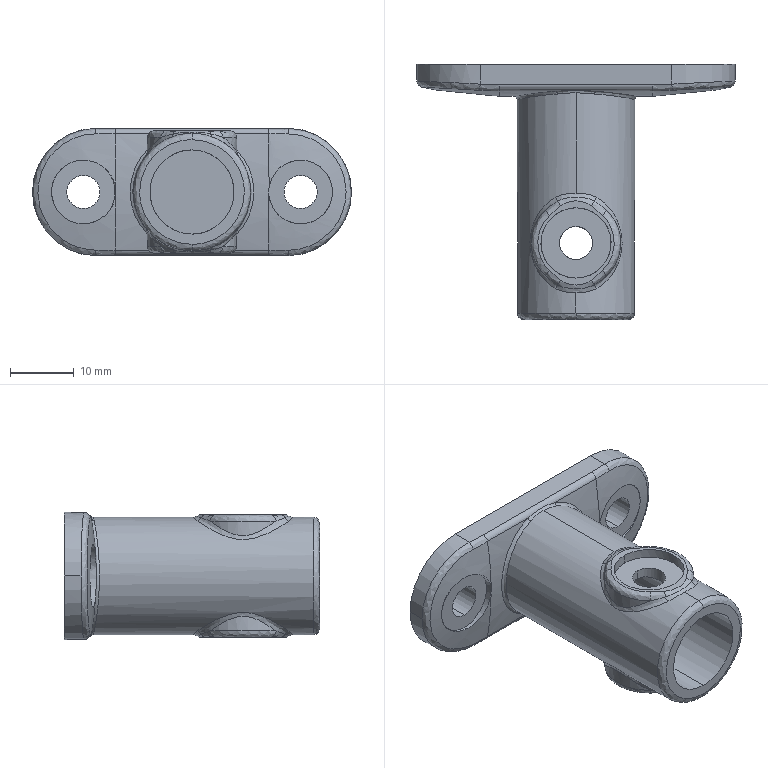Part | SolidWorks | features BaseBody 1 | 1 solid | 80 faces | box 50 x 40 x 19.965 mm | volume 7929 mm3 | spline 38 | cylinder 28 | plane 11 | cone 3 | commonest cylinder face diameters 5.2 x8 9.99 x4 11 x4 14 x4 2 x2 13.2 x2